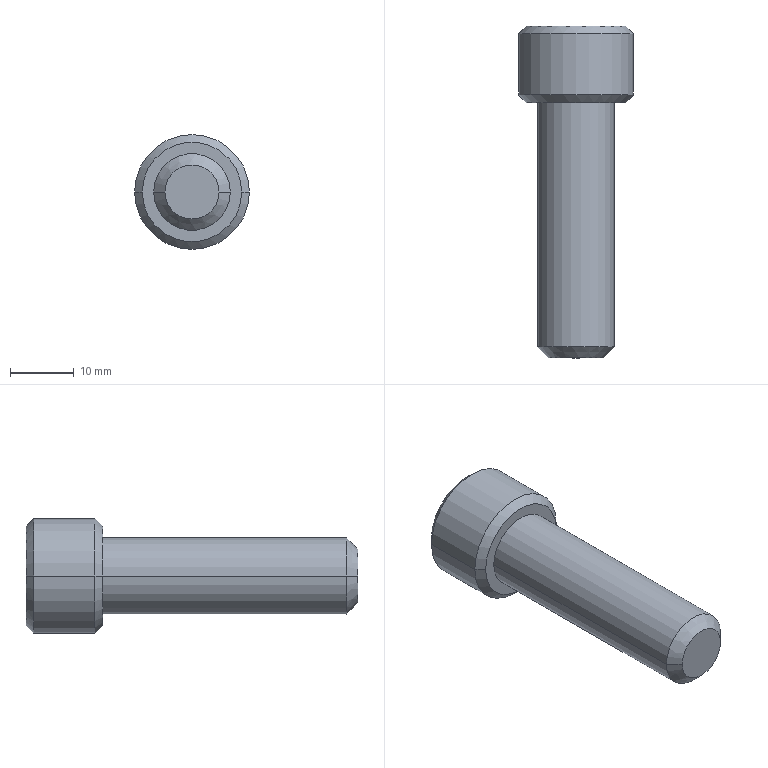Part | STEP file | BB62-M12-40L | 1 solid | 27 faces | box 18 x 52 x 18 mm | volume 6826 mm3 | plane 15 | cone 8 | cylinder 4 | commonest cylinder face diameters 12 x2 18 x2